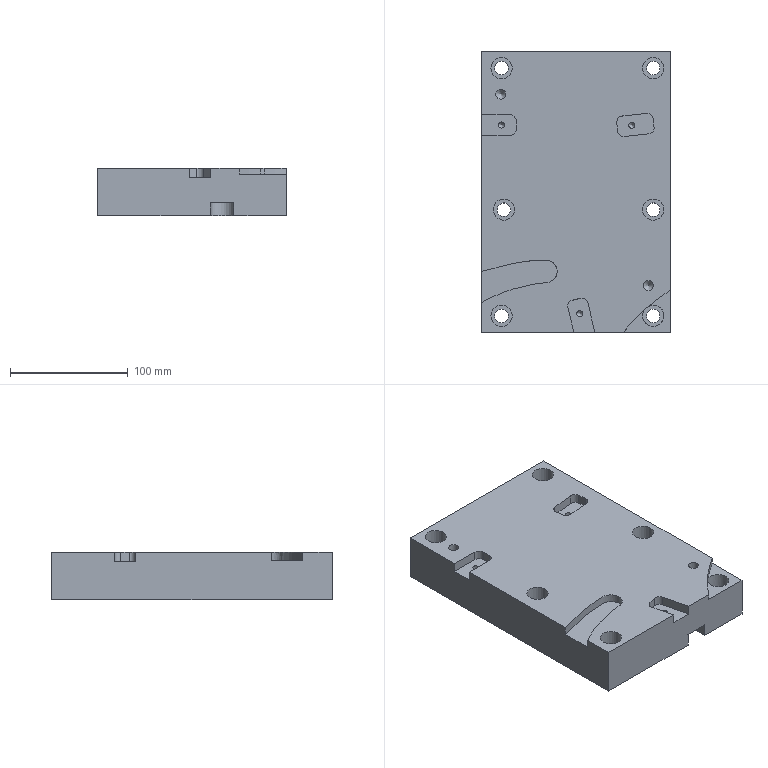Part | NX | features 23 2 | 1 solid | 78 faces | box 160 x 238 x 40 mm | volume 1408111 mm3 | plane 36 | cylinder 32 | spline 5 | cone 5 | commonest cylinder face diameters 10 x8 20 x7 11.5 x6 18 x6 5.2 x3 8.5 x2